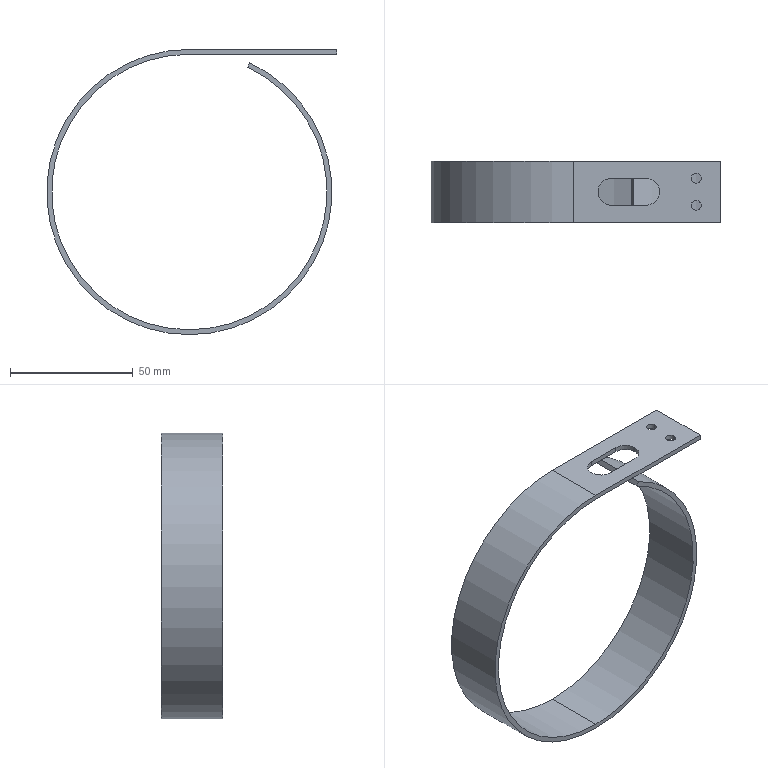Part | SolidWorks | features ExtruThin 1, ICE 1 | 1 solid | 19 faces | box 118 x 25 x 116 mm | volume 19115 mm3 | cylinder 11 | plane 8 | commonest cylinder face diameters 4 x4 11 x3 112 x2 116 x2
STEP:
#1=CARTESIAN_POINT('',(35.,0.,56.));
#2=VERTEX_POINT('',#1);
#3=CARTESIAN_POINT('',(29.5,5.5,56.));
#4=VERTEX_POINT('',#3);
#5=CARTESIAN_POINT('',(29.5,0.,56.));
#6=DIRECTION('',(0.,0.,1.));
#7=DIRECTION('',(1.,0.,0.));
#8=AXIS2_PLACEMENT_3D('',#5,#6,#7);
#9=CIRCLE('',#8,5.5);
#10=EDGE_CURVE('',#2,#4,#9,.T.);
#11=ORIENTED_EDGE('',*,*,#10,.F.);
#12=CARTESIAN_POINT('',(35.,0.,58.));
#13=VERTEX_POINT('',#12);
#14=CARTESIAN_POINT('',(35.,0.,56.));
#15=DIRECTION('',(0.,0.,1.));
#16=VECTOR('',#15,1000.);
#17=LINE('',#14,#16);
#18=EDGE_CURVE('',#2,#13,#17,.T.);
#19=ORIENTED_EDGE('',*,*,#18,.T.);
#20=CARTESIAN_POINT('',(29.5,5.5,58.));
#21=VERTEX_POINT('',#20);
#22=CARTESIAN_POINT('',(29.5,0.,58.));
#23=DIRECTION('',(0.,0.,1.));
#24=DIRECTION('',(1.,0.,0.));
#25=AXIS2_PLACEMENT_3D('',#22,#23,#24);
#26=CIRCLE('',#25,5.5);
#27=EDGE_CURVE('',#13,#21,#26,.T.);
#28=ORIENTED_EDGE('',*,*,#27,.T.);
#29=CARTESIAN_POINT('',(29.5,5.5,56.));
#30=DIRECTION('',(0.,0.,1.));
#31=VECTOR('',#30,1000.);
#32=LINE('',#29,#31);
#33=EDGE_CURVE('',#4,#21,#32,.T.);
#34=ORIENTED_EDGE('',*,*,#33,.F.);
#35=EDGE_LOOP('',(#11,#19,#28,#34));
#36=FACE_OUTER_BOUND('',#35,.T.);
#37=CARTESIAN_POINT('',(29.5,0.,56.));
#38=DIRECTION('',(0.,0.,1.));
#39=DIRECTION('',(1.,0.,0.));
#40=AXIS2_PLACEMENT_3D('',#37,#38,#39);
#41=CYLINDRICAL_SURFACE('',#40,5.5);
#42=ADVANCED_FACE('',(#36),#41,.F.);
#43=CARTESIAN_POINT('',(48.,5.5,56.));
#44=VERTEX_POINT('',#43);
#45=CARTESIAN_POINT('',(52.,5.5,56.));
#46=VERTEX_POINT('',#45);
#47=CARTESIAN_POINT('',(50.,5.5,56.));
#48=DIRECTION('',(0.,0.,1.));
#49=DIRECTION('',(1.,0.,0.));
#50=AXIS2_PLACEMENT_3D('',#47,#48,#49);
#51=CIRCLE('',#50,2.);
#52=EDGE_CURVE('',#44,#46,#51,.T.);
#53=ORIENTED_EDGE('',*,*,#52,.F.);
#54=CARTESIAN_POINT('',(48.,5.5,58.));
#55=VERTEX_POINT('',#54);
#56=CARTESIAN_POINT('',(48.,5.5,56.));
#57=DIRECTION('',(0.,0.,1.));
#58=VECTOR('',#57,1000.);
#59=LINE('',#56,#58);
#60=EDGE_CURVE('',#44,#55,#59,.T.);
#61=ORIENTED_EDGE('',*,*,#60,.T.);
#62=CARTESIAN_POINT('',(52.,5.5,58.));
#63=VERTEX_POINT('',#62);
#64=CARTESIAN_POINT('',(50.,5.5,58.));
#65=DIRECTION('',(0.,0.,1.));
#66=DIRECTION('',(1.,0.,0.));
#67=AXIS2_PLACEMENT_3D('',#64,#65,#66);
#68=CIRCLE('',#67,2.);
#69=EDGE_CURVE('',#55,#63,#68,.T.);
#70=ORIENTED_EDGE('',*,*,#69,.T.);
#71=CARTESIAN_POINT('',(52.,5.5,56.));
#72=DIRECTION('',(0.,0.,1.));
#73=VECTOR('',#72,1000.);
#74=LINE('',#71,#73);
#75=EDGE_CURVE('',#46,#63,#74,.T.);
#76=ORIENTED_EDGE('',*,*,#75,.F.);
#77=EDGE_LOOP('',(#53,#61,#70,#76));
#78=FACE_OUTER_BOUND('',#77,.T.);
#79=CARTESIAN_POINT('',(50.,5.5,56.));
#80=DIRECTION('',(0.,0.,1.));
#81=DIRECTION('',(1.,0.,0.));
#82=AXIS2_PLACEMENT_3D('',#79,#80,#81);
#83=CYLINDRICAL_SURFACE('',#82,2.);
#84=ADVANCED_FACE('',(#78),#83,.F.);
#85=CARTESIAN_POINT('',(48.,-5.5,56.));
#86=VERTEX_POINT('',#85);
#87=CARTESIAN_POINT('',(52.,-5.5,56.));
#88=VERTEX_POINT('',#87);
#89=CARTESIAN_POINT('',(50.,-5.5,56.));
#90=DIRECTION('',(0.,0.,1.));
#91=DIRECTION('',(-1.,0.,0.));
#92=AXIS2_PLACEMENT_3D('',#89,#90,#91);
#93=CIRCLE('',#92,2.);
#94=EDGE_CURVE('',#86,#88,#93,.T.);
#95=ORIENTED_EDGE('',*,*,#94,.F.);
#96=CARTESIAN_POINT('',(48.,-5.5,58.));
#97=VERTEX_POINT('',#96);
#98=CARTESIAN_POINT('',(48.,-5.5,56.));
#99=DIRECTION('',(0.,0.,1.));
#100=VECTOR('',#99,1000.);
#101=LINE('',#98,#100);
#102=EDGE_CURVE('',#86,#97,#101,.T.);
#103=ORIENTED_EDGE('',*,*,#102,.T.);
#104=CARTESIAN_POINT('',(52.,-5.5,58.));
#105=VERTEX_POINT('',#104);
#106=CARTESIAN_POINT('',(50.,-5.5,58.));
#107=DIRECTION('',(0.,0.,1.));
#108=DIRECTION('',(-1.,0.,0.));
#109=AXIS2_PLACEMENT_3D('',#106,#107,#108);
#110=CIRCLE('',#109,2.);
#111=EDGE_CURVE('',#97,#105,#110,.T.);
#112=ORIENTED_EDGE('',*,*,#111,.T.);
#113=CARTESIAN_POINT('',(52.,-5.5,56.));
#114=DIRECTION('',(0.,0.,1.));
#115=VECTOR('',#114,1000.);
#116=LINE('',#113,#115);
#117=EDGE_CURVE('',#88,#105,#116,.T.);
#118=ORIENTED_EDGE('',*,*,#117,.F.);
#119=EDGE_LOOP('',(#95,#103,#112,#118));
#120=FACE_OUTER_BOUND('',#119,.T.);
#121=CARTESIAN_POINT('',(50.,-5.5,56.));
#122=DIRECTION('',(0.,0.,1.));
#123=DIRECTION('',(1.,0.,0.));
#124=AXIS2_PLACEMENT_3D('',#121,#122,#123);
#125=CYLINDRICAL_SURFACE('',#124,2.);
#126=ADVANCED_FACE('',(#120),#125,.F.);
#127=CARTESIAN_POINT('',(0.,12.5,-58.));
#128=VERTEX_POINT('',#127);
#129=CARTESIAN_POINT('',(0.,12.5,58.));
#130=VERTEX_POINT('',#129);
#131=CARTESIAN_POINT('',(0.,12.5,0.));
#132=DIRECTION('',(0.,1.,0.));
#133=DIRECTION('',(1.,0.,0.));
#134=AXIS2_PLACEMENT_3D('',#131,#132,#133);
#135=CIRCLE('',#134,58.);
#136=EDGE_CURVE('',#128,#130,#135,.T.);
#137=ORIENTED_EDGE('',*,*,#136,.F.);
#138=CARTESIAN_POINT('',(0.,-12.5,-58.));
#139=VERTEX_POINT('',#138);
#140=CARTESIAN_POINT('',(0.,12.5,-58.));
#141=DIRECTION('',(0.,-1.,0.));
#142=VECTOR('',#141,1000.);
#143=LINE('',#140,#142);
#144=EDGE_CURVE('',#128,#139,#143,.T.);
#145=ORIENTED_EDGE('',*,*,#144,.T.);
#146=CARTESIAN_POINT('',(0.,-12.5,58.));
#147=VERTEX_POINT('',#146);
#148=CARTESIAN_POINT('',(0.,-12.5,0.));
#149=DIRECTION('',(0.,1.,0.));
#150=DIRECTION('',(1.,0.,0.));
#151=AXIS2_PLACEMENT_3D('',#148,#149,#150);
#152=CIRCLE('',#151,58.);
#153=EDGE_CURVE('',#139,#147,#152,.T.);
#154=ORIENTED_EDGE('',*,*,#153,.T.);
#155=CARTESIAN_POINT('',(0.,12.5,58.));
#156=DIRECTION('',(0.,-1.,0.));
#157=VECTOR('',#156,1000.);
#158=LINE('',#155,#157);
#159=EDGE_CURVE('',#130,#147,#158,.T.);
#160=ORIENTED_EDGE('',*,*,#159,.F.);
#161=EDGE_LOOP('',(#137,#145,#154,#160));
#162=FACE_OUTER_BOUND('',#161,.T.);
#163=CARTESIAN_POINT('',(0.,12.5,0.));
#164=DIRECTION('',(0.,-1.,0.));
#165=DIRECTION('',(0.,0.,-1.));
#166=AXIS2_PLACEMENT_3D('',#163,#164,#165);
#167=CYLINDRICAL_SURFACE('',#166,58.);
#168=ADVANCED_FACE('',(#162),#167,.T.);
#169=CARTESIAN_POINT('',(23.667,12.5,50.753));
#170=VERTEX_POINT('',#169);
#171=CARTESIAN_POINT('',(0.,12.5,-56.));
#172=VERTEX_POINT('',#171);
#173=CARTESIAN_POINT('',(0.,12.5,0.));
#174=DIRECTION('',(0.,1.,0.));
#175=DIRECTION('',(0.,0.,1.));
#176=AXIS2_PLACEMENT_3D('',#173,#174,#175);
#177=CIRCLE('',#176,56.);
#178=EDGE_CURVE('',#170,#172,#177,.T.);
#179=ORIENTED_EDGE('',*,*,#178,.T.);
#180=CARTESIAN_POINT('',(0.,-12.5,-56.));
#181=VERTEX_POINT('',#180);
#182=CARTESIAN_POINT('',(0.,12.5,-56.));
#183=DIRECTION('',(0.,-1.,0.));
#184=VECTOR('',#183,1000.);
#185=LINE('',#182,#184);
#186=EDGE_CURVE('',#172,#181,#185,.T.);
#187=ORIENTED_EDGE('',*,*,#186,.T.);
#188=CARTESIAN_POINT('',(23.667,-12.5,50.753));
#189=VERTEX_POINT('',#188);
#190=CARTESIAN_POINT('',(0.,-12.5,0.));
#191=DIRECTION('',(0.,1.,0.));
#192=DIRECTION('',(0.,0.,1.));
#193=AXIS2_PLACEMENT_3D('',#190,#191,#192);
#194=CIRCLE('',#193,56.);
#195=EDGE_CURVE('',#189,#181,#194,.T.);
#196=ORIENTED_EDGE('',*,*,#195,.F.);
#197=CARTESIAN_POINT('',(23.667,12.5,50.753));
#198=DIRECTION('',(0.,-1.,0.));
#199=VECTOR('',#198,1000.);
#200=LINE('',#197,#199);
#201=EDGE_CURVE('',#170,#189,#200,.T.);
#202=ORIENTED_EDGE('',*,*,#201,.F.);
#203=EDGE_LOOP('',(#179,#187,#196,#202));
#204=FACE_OUTER_BOUND('',#203,.T.);
#205=CARTESIAN_POINT('',(0.,12.5,0.));
#206=DIRECTION('',(0.,-1.,0.));
#207=DIRECTION('',(0.,0.,-1.));
#208=AXIS2_PLACEMENT_3D('',#205,#206,#207);
#209=CYLINDRICAL_SURFACE('',#208,56.);
#210=ADVANCED_FACE('',(#204),#209,.F.);
#211=CARTESIAN_POINT('',(15.5,-5.5,58.));
#212=VERTEX_POINT('',#211);
#213=CARTESIAN_POINT('',(29.5,-5.5,58.));
#214=VERTEX_POINT('',#213);
#215=CARTESIAN_POINT('',(15.5,-5.5,58.));
#216=DIRECTION('',(1.,0.,0.));
#217=VECTOR('',#216,1000.);
#218=LINE('',#215,#217);
#219=EDGE_CURVE('',#212,#214,#218,.T.);
#220=ORIENTED_EDGE('',*,*,#219,.F.);
#221=CARTESIAN_POINT('',(15.5,5.5,58.));
#222=VERTEX_POINT('',#221);
#223=CARTESIAN_POINT('',(15.5,0.,58.));
#224=DIRECTION('',(0.,0.,1.));
#225=DIRECTION('',(1.,0.,0.));
#226=AXIS2_PLACEMENT_3D('',#223,#224,#225);
#227=CIRCLE('',#226,5.5);
#228=EDGE_CURVE('',#222,#212,#227,.T.);
#229=ORIENTED_EDGE('',*,*,#228,.F.);
#230=CARTESIAN_POINT('',(15.5,5.5,58.));
#231=DIRECTION('',(-1.,0.,0.));
#232=VECTOR('',#231,1000.);
#233=LINE('',#230,#232);
#234=EDGE_CURVE('',#21,#222,#233,.T.);
#235=ORIENTED_EDGE('',*,*,#234,.F.);
#236=ORIENTED_EDGE('',*,*,#27,.F.);
#237=CARTESIAN_POINT('',(29.5,0.,58.));
#238=DIRECTION('',(0.,0.,1.));
#239=DIRECTION('',(1.,0.,0.));
#240=AXIS2_PLACEMENT_3D('',#237,#238,#239);
#241=CIRCLE('',#240,5.5);
#242=EDGE_CURVE('',#214,#13,#241,.T.);
#243=ORIENTED_EDGE('',*,*,#242,.F.);
#244=EDGE_LOOP('',(#220,#229,#235,#236,#243));
#245=FACE_BOUND('',#244,.T.);
#246=CARTESIAN_POINT('',(50.,5.5,58.));
#247=DIRECTION('',(0.,0.,1.));
#248=DIRECTION('',(1.,0.,0.));
#249=AXIS2_PLACEMENT_3D('',#246,#247,#248);
#250=CIRCLE('',#249,2.);
#251=EDGE_CURVE('',#63,#55,#250,.T.);
#252=ORIENTED_EDGE('',*,*,#251,.F.);
#253=ORIENTED_EDGE('',*,*,#69,.F.);
#254=EDGE_LOOP('',(#252,#253));
#255=FACE_BOUND('',#254,.T.);
#256=CARTESIAN_POINT('',(50.,-5.5,58.));
#257=DIRECTION('',(0.,0.,1.));
#258=DIRECTION('',(-1.,0.,0.));
#259=AXIS2_PLACEMENT_3D('',#256,#257,#258);
#260=CIRCLE('',#259,2.);
#261=EDGE_CURVE('',#105,#97,#260,.T.);
#262=ORIENTED_EDGE('',*,*,#261,.F.);
#263=ORIENTED_EDGE('',*,*,#111,.F.);
#264=EDGE_LOOP('',(#262,#263));
#265=FACE_BOUND('',#264,.T.);
#266=CARTESIAN_POINT('',(60.,-12.5,58.));
#267=VERTEX_POINT('',#266);
#268=CARTESIAN_POINT('',(0.,-12.5,58.));
#269=DIRECTION('',(1.,0.,0.));
#270=VECTOR('',#269,1000.);
#271=LINE('',#268,#270);
#272=EDGE_CURVE('',#147,#267,#271,.T.);
#273=ORIENTED_EDGE('',*,*,#272,.T.);
#274=CARTESIAN_POINT('',(60.,12.5,58.));
#275=VERTEX_POINT('',#274);
#276=CARTESIAN_POINT('',(60.,12.5,58.));
#277=DIRECTION('',(0.,-1.,0.));
#278=VECTOR('',#277,1000.);
#279=LINE('',#276,#278);
#280=EDGE_CURVE('',#275,#267,#279,.T.);
#281=ORIENTED_EDGE('',*,*,#280,.F.);
#282=CARTESIAN_POINT('',(0.,12.5,58.));
#283=DIRECTION('',(1.,0.,0.));
#284=VECTOR('',#283,1000.);
#285=LINE('',#282,#284);
#286=EDGE_CURVE('',#130,#275,#285,.T.);
#287=ORIENTED_EDGE('',*,*,#286,.F.);
#288=ORIENTED_EDGE('',*,*,#159,.T.);
#289=EDGE_LOOP('',(#273,#281,#287,#288));
#290=FACE_OUTER_BOUND('',#289,.T.);
#291=CARTESIAN_POINT('',(0.,12.5,58.));
#292=DIRECTION('',(0.,0.,-1.));
#293=DIRECTION('',(-1.,0.,0.));
#294=AXIS2_PLACEMENT_3D('',#291,#292,#293);
#295=PLANE('',#294);
#296=ADVANCED_FACE('',(#245,#255,#265,#290),#295,.F.);
#297=CARTESIAN_POINT('',(60.,-12.5,56.));
#298=VERTEX_POINT('',#297);
#299=CARTESIAN_POINT('',(60.,-12.5,56.));
#300=DIRECTION('',(0.,0.,1.));
#301=VECTOR('',#300,1000.);
#302=LINE('',#299,#301);
#303=EDGE_CURVE('',#298,#267,#302,.T.);
#304=ORIENTED_EDGE('',*,*,#303,.F.);
#305=CARTESIAN_POINT('',(60.,12.5,56.));
#306=VERTEX_POINT('',#305);
#307=CARTESIAN_POINT('',(60.,12.5,56.));
#308=DIRECTION('',(0.,-1.,0.));
#309=VECTOR('',#308,1000.);
#310=LINE('',#307,#309);
#311=EDGE_CURVE('',#306,#298,#310,.T.);
#312=ORIENTED_EDGE('',*,*,#311,.F.);
#313=CARTESIAN_POINT('',(60.,12.5,56.));
#314=DIRECTION('',(0.,0.,1.));
#315=VECTOR('',#314,1000.);
#316=LINE('',#313,#315);
#317=EDGE_CURVE('',#306,#275,#316,.T.);
#318=ORIENTED_EDGE('',*,*,#317,.T.);
#319=ORIENTED_EDGE('',*,*,#280,.T.);
#320=EDGE_LOOP('',(#304,#312,#318,#319));
#321=FACE_OUTER_BOUND('',#320,.T.);
#322=CARTESIAN_POINT('',(60.,12.5,56.));
#323=DIRECTION('',(1.,0.,0.));
#324=DIRECTION('',(0.,0.,-1.));
#325=AXIS2_PLACEMENT_3D('',#322,#323,#324);
#326=PLANE('',#325);
#327=ADVANCED_FACE('',(#321),#326,.T.);
#328=CARTESIAN_POINT('',(15.5,5.5,56.));
#329=VERTEX_POINT('',#328);
#330=CARTESIAN_POINT('',(15.5,-5.5,56.));
#331=VERTEX_POINT('',#330);
#332=CARTESIAN_POINT('',(15.5,0.,56.));
#333=DIRECTION('',(0.,0.,1.));
#334=DIRECTION('',(1.,0.,0.));
#335=AXIS2_PLACEMENT_3D('',#332,#333,#334);
#336=CIRCLE('',#335,5.5);
#337=EDGE_CURVE('',#329,#331,#336,.T.);
#338=ORIENTED_EDGE('',*,*,#337,.T.);
#339=CARTESIAN_POINT('',(29.5,-5.5,56.));
#340=VERTEX_POINT('',#339);
#341=CARTESIAN_POINT('',(15.5,-5.5,56.));
#342=DIRECTION('',(1.,0.,0.));
#343=VECTOR('',#342,1000.);
#344=LINE('',#341,#343);
#345=EDGE_CURVE('',#331,#340,#344,.T.);
#346=ORIENTED_EDGE('',*,*,#345,.T.);
#347=CARTESIAN_POINT('',(29.5,0.,56.));
#348=DIRECTION('',(0.,0.,1.));
#349=DIRECTION('',(1.,0.,0.));
#350=AXIS2_PLACEMENT_3D('',#347,#348,#349);
#351=CIRCLE('',#350,5.5);
#352=EDGE_CURVE('',#340,#2,#351,.T.);
#353=ORIENTED_EDGE('',*,*,#352,.T.);
#354=ORIENTED_EDGE('',*,*,#10,.T.);
#355=CARTESIAN_POINT('',(15.5,5.5,56.));
#356=DIRECTION('',(-1.,0.,0.));
#357=VECTOR('',#356,1000.);
#358=LINE('',#355,#357);
#359=EDGE_CURVE('',#4,#329,#358,.T.);
#360=ORIENTED_EDGE('',*,*,#359,.T.);
#361=EDGE_LOOP('',(#338,#346,#353,#354,#360));
#362=FACE_BOUND('',#361,.T.);
#363=CARTESIAN_POINT('',(50.,5.5,56.));
#364=DIRECTION('',(0.,0.,1.));
#365=DIRECTION('',(1.,0.,0.));
#366=AXIS2_PLACEMENT_3D('',#363,#364,#365);
#367=CIRCLE('',#366,2.);
#368=EDGE_CURVE('',#46,#44,#367,.T.);
#369=ORIENTED_EDGE('',*,*,#368,.T.);
#370=ORIENTED_EDGE('',*,*,#52,.T.);
#371=EDGE_LOOP('',(#369,#370));
#372=FACE_BOUND('',#371,.T.);
#373=CARTESIAN_POINT('',(50.,-5.5,56.));
#374=DIRECTION('',(0.,0.,1.));
#375=DIRECTION('',(-1.,0.,0.));
#376=AXIS2_PLACEMENT_3D('',#373,#374,#375);
#377=CIRCLE('',#376,2.);
#378=EDGE_CURVE('',#88,#86,#377,.T.);
#379=ORIENTED_EDGE('',*,*,#378,.T.);
#380=ORIENTED_EDGE('',*,*,#94,.T.);
#381=EDGE_LOOP('',(#379,#380));
#382=FACE_BOUND('',#381,.T.);
#383=CARTESIAN_POINT('',(0.,-12.5,56.));
#384=VERTEX_POINT('',#383);
#385=CARTESIAN_POINT('',(0.,-12.5,56.));
#386=DIRECTION('',(1.,0.,0.));
#387=VECTOR('',#386,1000.);
#388=LINE('',#385,#387);
#389=EDGE_CURVE('',#384,#298,#388,.T.);
#390=ORIENTED_EDGE('',*,*,#389,.F.);
#391=CARTESIAN_POINT('',(0.,12.5,56.));
#392=VERTEX_POINT('',#391);
#393=CARTESIAN_POINT('',(0.,12.5,56.));
#394=DIRECTION('',(0.,-1.,0.));
#395=VECTOR('',#394,1000.);
#396=LINE('',#393,#395);
#397=EDGE_CURVE('',#392,#384,#396,.T.);
#398=ORIENTED_EDGE('',*,*,#397,.F.);
#399=CARTESIAN_POINT('',(0.,12.5,56.));
#400=DIRECTION('',(1.,0.,0.));
#401=VECTOR('',#400,1000.);
#402=LINE('',#399,#401);
#403=EDGE_CURVE('',#392,#306,#402,.T.);
#404=ORIENTED_EDGE('',*,*,#403,.T.);
#405=ORIENTED_EDGE('',*,*,#311,.T.);
#406=EDGE_LOOP('',(#390,#398,#404,#405));
#407=FACE_OUTER_BOUND('',#406,.T.);
#408=CARTESIAN_POINT('',(0.,12.5,56.));
#409=DIRECTION('',(0.,0.,-1.));
#410=DIRECTION('',(-1.,0.,0.));
#411=AXIS2_PLACEMENT_3D('',#408,#409,#410);
#412=PLANE('',#411);
#413=ADVANCED_FACE('',(#362,#372,#382,#407),#412,.T.);
#414=ORIENTED_EDGE('',*,*,#186,.F.);
#415=CARTESIAN_POINT('',(0.,12.5,0.));
#416=DIRECTION('',(0.,1.,0.));
#417=DIRECTION('',(0.,0.,1.));
#418=AXIS2_PLACEMENT_3D('',#415,#416,#417);
#419=CIRCLE('',#418,56.);
#420=EDGE_CURVE('',#172,#392,#419,.T.);
#421=ORIENTED_EDGE('',*,*,#420,.T.);
#422=ORIENTED_EDGE('',*,*,#397,.T.);
#423=CARTESIAN_POINT('',(0.,-12.5,0.));
#424=DIRECTION('',(0.,1.,0.));
#425=DIRECTION('',(0.,0.,1.));
#426=AXIS2_PLACEMENT_3D('',#423,#424,#425);
#427=CIRCLE('',#426,56.);
#428=EDGE_CURVE('',#181,#384,#427,.T.);
#429=ORIENTED_EDGE('',*,*,#428,.F.);
#430=EDGE_LOOP('',(#414,#421,#422,#429));
#431=FACE_OUTER_BOUND('',#430,.T.);
#432=CARTESIAN_POINT('',(0.,12.5,0.));
#433=DIRECTION('',(0.,-1.,0.));
#434=DIRECTION('',(0.,0.,-1.));
#435=AXIS2_PLACEMENT_3D('',#432,#433,#434);
#436=CYLINDRICAL_SURFACE('',#435,56.);
#437=ADVANCED_FACE('',(#431),#436,.F.);
#438=CARTESIAN_POINT('',(24.512,-12.5,52.566));
#439=VERTEX_POINT('',#438);
#440=CARTESIAN_POINT('',(24.512,-12.5,52.566));
#441=DIRECTION('',(-0.4226,0.,-0.9063));
#442=VECTOR('',#441,1000.);
#443=LINE('',#440,#442);
#444=EDGE_CURVE('',#439,#189,#443,.T.);
#445=ORIENTED_EDGE('',*,*,#444,.F.);
#446=CARTESIAN_POINT('',(24.512,12.5,52.566));
#447=VERTEX_POINT('',#446);
#448=CARTESIAN_POINT('',(24.512,12.5,52.566));
#449=DIRECTION('',(0.,-1.,0.));
#450=VECTOR('',#449,1000.);
#451=LINE('',#448,#450);
#452=EDGE_CURVE('',#447,#439,#451,.T.);
#453=ORIENTED_EDGE('',*,*,#452,.F.);
#454=CARTESIAN_POINT('',(24.512,12.5,52.566));
#455=DIRECTION('',(-0.4226,0.,-0.9063));
#456=VECTOR('',#455,1000.);
#457=LINE('',#454,#456);
#458=EDGE_CURVE('',#447,#170,#457,.T.);
#459=ORIENTED_EDGE('',*,*,#458,.T.);
#460=ORIENTED_EDGE('',*,*,#201,.T.);
#461=EDGE_LOOP('',(#445,#453,#459,#460));
#462=FACE_OUTER_BOUND('',#461,.T.);
#463=CARTESIAN_POINT('',(24.512,12.5,52.566));
#464=DIRECTION('',(-0.9063,0.,0.4226));
#465=DIRECTION('',(0.4226,0.,0.9063));
#466=AXIS2_PLACEMENT_3D('',#463,#464,#465);
#467=PLANE('',#466);
#468=ADVANCED_FACE('',(#462),#467,.T.);
#469=ORIENTED_EDGE('',*,*,#144,.F.);
#470=CARTESIAN_POINT('',(0.,12.5,0.));
#471=DIRECTION('',(0.,1.,0.));
#472=DIRECTION('',(1.,0.,0.));
#473=AXIS2_PLACEMENT_3D('',#470,#471,#472);
#474=CIRCLE('',#473,58.);
#475=EDGE_CURVE('',#447,#128,#474,.T.);
#476=ORIENTED_EDGE('',*,*,#475,.F.);
#477=ORIENTED_EDGE('',*,*,#452,.T.);
#478=CARTESIAN_POINT('',(0.,-12.5,0.));
#479=DIRECTION('',(0.,1.,0.));
#480=DIRECTION('',(1.,0.,0.));
#481=AXIS2_PLACEMENT_3D('',#478,#479,#480);
#482=CIRCLE('',#481,58.);
#483=EDGE_CURVE('',#439,#139,#482,.T.);
#484=ORIENTED_EDGE('',*,*,#483,.T.);
#485=EDGE_LOOP('',(#469,#476,#477,#484));
#486=FACE_OUTER_BOUND('',#485,.T.);
#487=CARTESIAN_POINT('',(0.,12.5,0.));
#488=DIRECTION('',(0.,-1.,0.));
#489=DIRECTION('',(0.,0.,-1.));
#490=AXIS2_PLACEMENT_3D('',#487,#488,#489);
#491=CYLINDRICAL_SURFACE('',#490,58.);
#492=ADVANCED_FACE('',(#486),#491,.T.);
#493=ORIENTED_EDGE('',*,*,#286,.T.);
#494=ORIENTED_EDGE('',*,*,#317,.F.);
#495=ORIENTED_EDGE('',*,*,#403,.F.);
#496=ORIENTED_EDGE('',*,*,#420,.F.);
#497=ORIENTED_EDGE('',*,*,#178,.F.);
#498=ORIENTED_EDGE('',*,*,#458,.F.);
#499=ORIENTED_EDGE('',*,*,#475,.T.);
#500=ORIENTED_EDGE('',*,*,#136,.T.);
#501=EDGE_LOOP('',(#493,#494,#495,#496,#497,#498,#499,#500));
#502=FACE_OUTER_BOUND('',#501,.T.);
#503=CARTESIAN_POINT('',(0.,12.5,0.));
#504=DIRECTION('',(0.,1.,0.));
#505=DIRECTION('',(1.,0.,0.));
#506=AXIS2_PLACEMENT_3D('',#503,#504,#505);
#507=PLANE('',#506);
#508=ADVANCED_FACE('',(#502),#507,.T.);
#509=ORIENTED_EDGE('',*,*,#272,.F.);
#510=ORIENTED_EDGE('',*,*,#153,.F.);
#511=ORIENTED_EDGE('',*,*,#483,.F.);
#512=ORIENTED_EDGE('',*,*,#444,.T.);
#513=ORIENTED_EDGE('',*,*,#195,.T.);
#514=ORIENTED_EDGE('',*,*,#428,.T.);
#515=ORIENTED_EDGE('',*,*,#389,.T.);
#516=ORIENTED_EDGE('',*,*,#303,.T.);
#517=EDGE_LOOP('',(#509,#510,#511,#512,#513,#514,#515,#516));
#518=FACE_OUTER_BOUND('',#517,.T.);
#519=CARTESIAN_POINT('',(0.,-12.5,0.));
#520=DIRECTION('',(0.,1.,0.));
#521=DIRECTION('',(1.,0.,0.));
#522=AXIS2_PLACEMENT_3D('',#519,#520,#521);
#523=PLANE('',#522);
#524=ADVANCED_FACE('',(#518),#523,.F.);
#525=ORIENTED_EDGE('',*,*,#102,.F.);
#526=ORIENTED_EDGE('',*,*,#378,.F.);
#527=ORIENTED_EDGE('',*,*,#117,.T.);
#528=ORIENTED_EDGE('',*,*,#261,.T.);
#529=EDGE_LOOP('',(#525,#526,#527,#528));
#530=FACE_OUTER_BOUND('',#529,.T.);
#531=CARTESIAN_POINT('',(50.,-5.5,56.));
#532=DIRECTION('',(0.,0.,1.));
#533=DIRECTION('',(1.,0.,0.));
#534=AXIS2_PLACEMENT_3D('',#531,#532,#533);
#535=CYLINDRICAL_SURFACE('',#534,2.);
#536=ADVANCED_FACE('',(#530),#535,.F.);
#537=ORIENTED_EDGE('',*,*,#60,.F.);
#538=ORIENTED_EDGE('',*,*,#368,.F.);
#539=ORIENTED_EDGE('',*,*,#75,.T.);
#540=ORIENTED_EDGE('',*,*,#251,.T.);
#541=EDGE_LOOP('',(#537,#538,#539,#540));
#542=FACE_OUTER_BOUND('',#541,.T.);
#543=CARTESIAN_POINT('',(50.,5.5,56.));
#544=DIRECTION('',(0.,0.,1.));
#545=DIRECTION('',(1.,0.,0.));
#546=AXIS2_PLACEMENT_3D('',#543,#544,#545);
#547=CYLINDRICAL_SURFACE('',#546,2.);
#548=ADVANCED_FACE('',(#542),#547,.F.);
#549=ORIENTED_EDGE('',*,*,#228,.T.);
#550=CARTESIAN_POINT('',(15.5,-5.5,56.));
#551=DIRECTION('',(0.,0.,1.));
#552=VECTOR('',#551,1000.);
#553=LINE('',#550,#552);
#554=EDGE_CURVE('',#331,#212,#553,.T.);
#555=ORIENTED_EDGE('',*,*,#554,.F.);
#556=ORIENTED_EDGE('',*,*,#337,.F.);
#557=CARTESIAN_POINT('',(15.5,5.5,56.));
#558=DIRECTION('',(0.,0.,1.));
#559=VECTOR('',#558,1000.);
#560=LINE('',#557,#559);
#561=EDGE_CURVE('',#329,#222,#560,.T.);
#562=ORIENTED_EDGE('',*,*,#561,.T.);
#563=EDGE_LOOP('',(#549,#555,#556,#562));
#564=FACE_OUTER_BOUND('',#563,.T.);
#565=CARTESIAN_POINT('',(15.5,0.,56.));
#566=DIRECTION('',(0.,0.,1.));
#567=DIRECTION('',(1.,0.,0.));
#568=AXIS2_PLACEMENT_3D('',#565,#566,#567);
#569=CYLINDRICAL_SURFACE('',#568,5.5);
#570=ADVANCED_FACE('',(#564),#569,.F.);
#571=ORIENTED_EDGE('',*,*,#234,.T.);
#572=ORIENTED_EDGE('',*,*,#561,.F.);
#573=ORIENTED_EDGE('',*,*,#359,.F.);
#574=ORIENTED_EDGE('',*,*,#33,.T.);
#575=EDGE_LOOP('',(#571,#572,#573,#574));
#576=FACE_OUTER_BOUND('',#575,.T.);
#577=CARTESIAN_POINT('',(15.5,5.5,56.));
#578=DIRECTION('',(0.,1.,0.));
#579=DIRECTION('',(0.,0.,1.));
#580=AXIS2_PLACEMENT_3D('',#577,#578,#579);
#581=PLANE('',#580);
#582=ADVANCED_FACE('',(#576),#581,.F.);
#583=ORIENTED_EDGE('',*,*,#18,.F.);
#584=ORIENTED_EDGE('',*,*,#352,.F.);
#585=CARTESIAN_POINT('',(29.5,-5.5,56.));
#586=DIRECTION('',(0.,0.,1.));
#587=VECTOR('',#586,1000.);
#588=LINE('',#585,#587);
#589=EDGE_CURVE('',#340,#214,#588,.T.);
#590=ORIENTED_EDGE('',*,*,#589,.T.);
#591=ORIENTED_EDGE('',*,*,#242,.T.);
#592=EDGE_LOOP('',(#583,#584,#590,#591));
#593=FACE_OUTER_BOUND('',#592,.T.);
#594=CARTESIAN_POINT('',(29.5,0.,56.));
#595=DIRECTION('',(0.,0.,1.));
#596=DIRECTION('',(1.,0.,0.));
#597=AXIS2_PLACEMENT_3D('',#594,#595,#596);
#598=CYLINDRICAL_SURFACE('',#597,5.5);
#599=ADVANCED_FACE('',(#593),#598,.F.);
#600=ORIENTED_EDGE('',*,*,#219,.T.);
#601=ORIENTED_EDGE('',*,*,#589,.F.);
#602=ORIENTED_EDGE('',*,*,#345,.F.);
#603=ORIENTED_EDGE('',*,*,#554,.T.);
#604=EDGE_LOOP('',(#600,#601,#602,#603));
#605=FACE_OUTER_BOUND('',#604,.T.);
#606=CARTESIAN_POINT('',(15.5,-5.5,56.));
#607=DIRECTION('',(0.,-1.,0.));
#608=DIRECTION('',(0.,0.,-1.));
#609=AXIS2_PLACEMENT_3D('',#606,#607,#608);
#610=PLANE('',#609);
#611=ADVANCED_FACE('',(#605),#610,.F.);
#612=CLOSED_SHELL('',(#42,#84,#126,#168,#210,#296,#327,#413,#437,#468,#492,#508,#524,#536,#548,#570,#582,#599,#611));
#613=MANIFOLD_SOLID_BREP('',#612);
#614=CARTESIAN_POINT('',(0.,0.,0.));
#615=DIRECTION('',(0.,0.,1.));
#616=DIRECTION('',(1.,0.,0.));
#617=AXIS2_PLACEMENT_3D('',#614,#615,#616);
#618=(LENGTH_UNIT()NAMED_UNIT(*)SI_UNIT(.MILLI.,.METRE.));
#619=UNCERTAINTY_MEASURE_WITH_UNIT(LENGTH_MEASURE(0.00001),#618,'','');
#620=(NAMED_UNIT(*)PLANE_ANGLE_UNIT()SI_UNIT($,.RADIAN.));
#621=(NAMED_UNIT(*)SI_UNIT($,.STERADIAN.)SOLID_ANGLE_UNIT());
#622=(GEOMETRIC_REPRESENTATION_CONTEXT(3)GLOBAL_UNCERTAINTY_ASSIGNED_CONTEXT((#619))GLOBAL_UNIT_ASSIGNED_CONTEXT((#618,#620,#621))REPRESENTATION_CONTEXT('',''));
#623=ADVANCED_BREP_SHAPE_REPRESENTATION('',(#613,#617),#622);